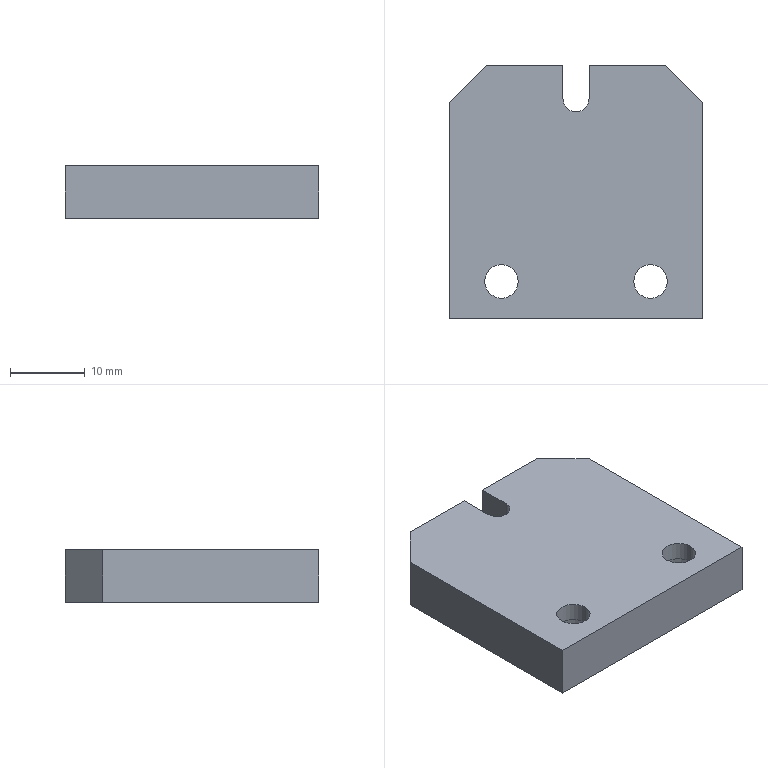Part | STEP file | 11-FG-B02011 | 1 solid | 22 faces | box 34 x 34 x 7 mm | volume 7241 mm3 | plane 13 | cylinder 9 | commonest cylinder face diameters 4.5 x4 8 x4 3.5 x1
STEP:
#1=CARTESIAN_POINT('',(11.,5.,4.5));
#2=VERTEX_POINT('',#1);
#3=CARTESIAN_POINT('',(3.,5.,4.5));
#4=VERTEX_POINT('',#3);
#5=CARTESIAN_POINT('',(7.,5.,4.5));
#6=DIRECTION('',(0.,0.,-1.));
#7=DIRECTION('',(-1.,0.,0.));
#8=AXIS2_PLACEMENT_3D('',#5,#6,#7);
#9=CIRCLE('',#8,4.);
#10=EDGE_CURVE('',#2,#4,#9,.T.);
#11=ORIENTED_EDGE('',*,*,#10,.F.);
#12=CARTESIAN_POINT('',(11.,5.,0.));
#13=VERTEX_POINT('',#12);
#14=CARTESIAN_POINT('',(11.,5.,4.5));
#15=DIRECTION('',(0.,0.,-1.));
#16=VECTOR('',#15,1000.);
#17=LINE('',#14,#16);
#18=EDGE_CURVE('',#2,#13,#17,.T.);
#19=ORIENTED_EDGE('',*,*,#18,.T.);
#20=CARTESIAN_POINT('',(3.,5.,0.));
#21=VERTEX_POINT('',#20);
#22=CARTESIAN_POINT('',(7.,5.,0.));
#23=DIRECTION('',(0.,0.,-1.));
#24=DIRECTION('',(-1.,0.,0.));
#25=AXIS2_PLACEMENT_3D('',#22,#23,#24);
#26=CIRCLE('',#25,4.);
#27=EDGE_CURVE('',#13,#21,#26,.T.);
#28=ORIENTED_EDGE('',*,*,#27,.T.);
#29=CARTESIAN_POINT('',(3.,5.,4.5));
#30=DIRECTION('',(0.,0.,-1.));
#31=VECTOR('',#30,1000.);
#32=LINE('',#29,#31);
#33=EDGE_CURVE('',#4,#21,#32,.T.);
#34=ORIENTED_EDGE('',*,*,#33,.F.);
#35=EDGE_LOOP('',(#11,#19,#28,#34));
#36=FACE_OUTER_BOUND('',#35,.T.);
#37=CARTESIAN_POINT('',(7.,5.,4.5));
#38=DIRECTION('',(0.,0.,-1.));
#39=DIRECTION('',(-1.,0.,0.));
#40=AXIS2_PLACEMENT_3D('',#37,#38,#39);
#41=CYLINDRICAL_SURFACE('',#40,4.);
#42=ADVANCED_FACE('',(#36),#41,.F.);
#43=CARTESIAN_POINT('',(31.,5.,4.5));
#44=VERTEX_POINT('',#43);
#45=CARTESIAN_POINT('',(23.,5.,4.5));
#46=VERTEX_POINT('',#45);
#47=CARTESIAN_POINT('',(27.,5.,4.5));
#48=DIRECTION('',(0.,0.,-1.));
#49=DIRECTION('',(-1.,0.,0.));
#50=AXIS2_PLACEMENT_3D('',#47,#48,#49);
#51=CIRCLE('',#50,4.);
#52=EDGE_CURVE('',#44,#46,#51,.T.);
#53=ORIENTED_EDGE('',*,*,#52,.F.);
#54=CARTESIAN_POINT('',(31.,5.,0.));
#55=VERTEX_POINT('',#54);
#56=CARTESIAN_POINT('',(31.,5.,4.5));
#57=DIRECTION('',(0.,0.,-1.));
#58=VECTOR('',#57,1000.);
#59=LINE('',#56,#58);
#60=EDGE_CURVE('',#44,#55,#59,.T.);
#61=ORIENTED_EDGE('',*,*,#60,.T.);
#62=CARTESIAN_POINT('',(23.,5.,0.));
#63=VERTEX_POINT('',#62);
#64=CARTESIAN_POINT('',(27.,5.,0.));
#65=DIRECTION('',(0.,0.,-1.));
#66=DIRECTION('',(-1.,0.,0.));
#67=AXIS2_PLACEMENT_3D('',#64,#65,#66);
#68=CIRCLE('',#67,4.);
#69=EDGE_CURVE('',#55,#63,#68,.T.);
#70=ORIENTED_EDGE('',*,*,#69,.T.);
#71=CARTESIAN_POINT('',(23.,5.,4.5));
#72=DIRECTION('',(0.,0.,-1.));
#73=VECTOR('',#72,1000.);
#74=LINE('',#71,#73);
#75=EDGE_CURVE('',#46,#63,#74,.T.);
#76=ORIENTED_EDGE('',*,*,#75,.F.);
#77=EDGE_LOOP('',(#53,#61,#70,#76));
#78=FACE_OUTER_BOUND('',#77,.T.);
#79=CARTESIAN_POINT('',(27.,5.,4.5));
#80=DIRECTION('',(0.,0.,-1.));
#81=DIRECTION('',(-1.,0.,0.));
#82=AXIS2_PLACEMENT_3D('',#79,#80,#81);
#83=CYLINDRICAL_SURFACE('',#82,4.);
#84=ADVANCED_FACE('',(#78),#83,.F.);
#85=CARTESIAN_POINT('',(24.75,5.,4.5));
#86=VERTEX_POINT('',#85);
#87=CARTESIAN_POINT('',(29.25,5.,4.5));
#88=VERTEX_POINT('',#87);
#89=CARTESIAN_POINT('',(27.,5.,4.5));
#90=DIRECTION('',(0.,0.,1.));
#91=DIRECTION('',(-1.,0.,0.));
#92=AXIS2_PLACEMENT_3D('',#89,#90,#91);
#93=CIRCLE('',#92,2.25);
#94=EDGE_CURVE('',#86,#88,#93,.T.);
#95=ORIENTED_EDGE('',*,*,#94,.F.);
#96=CARTESIAN_POINT('',(24.75,5.,7.));
#97=VERTEX_POINT('',#96);
#98=CARTESIAN_POINT('',(24.75,5.,0.));
#99=DIRECTION('',(0.,0.,1.));
#100=VECTOR('',#99,1000.);
#101=LINE('',#98,#100);
#102=EDGE_CURVE('',#86,#97,#101,.T.);
#103=ORIENTED_EDGE('',*,*,#102,.T.);
#104=CARTESIAN_POINT('',(29.25,5.,7.));
#105=VERTEX_POINT('',#104);
#106=CARTESIAN_POINT('',(27.,5.,7.));
#107=DIRECTION('',(0.,0.,1.));
#108=DIRECTION('',(1.,0.,0.));
#109=AXIS2_PLACEMENT_3D('',#106,#107,#108);
#110=CIRCLE('',#109,2.25);
#111=EDGE_CURVE('',#97,#105,#110,.T.);
#112=ORIENTED_EDGE('',*,*,#111,.T.);
#113=CARTESIAN_POINT('',(29.25,5.,0.));
#114=DIRECTION('',(0.,0.,1.));
#115=VECTOR('',#114,1000.);
#116=LINE('',#113,#115);
#117=EDGE_CURVE('',#88,#105,#116,.T.);
#118=ORIENTED_EDGE('',*,*,#117,.F.);
#119=EDGE_LOOP('',(#95,#103,#112,#118));
#120=FACE_OUTER_BOUND('',#119,.T.);
#121=CARTESIAN_POINT('',(27.,5.,0.));
#122=DIRECTION('',(0.,0.,1.));
#123=DIRECTION('',(1.,0.,0.));
#124=AXIS2_PLACEMENT_3D('',#121,#122,#123);
#125=CYLINDRICAL_SURFACE('',#124,2.25);
#126=ADVANCED_FACE('',(#120),#125,.F.);
#127=CARTESIAN_POINT('',(4.75,5.,4.5));
#128=VERTEX_POINT('',#127);
#129=CARTESIAN_POINT('',(9.25,5.,4.5));
#130=VERTEX_POINT('',#129);
#131=CARTESIAN_POINT('',(7.,5.,4.5));
#132=DIRECTION('',(0.,0.,1.));
#133=DIRECTION('',(-1.,0.,0.));
#134=AXIS2_PLACEMENT_3D('',#131,#132,#133);
#135=CIRCLE('',#134,2.25);
#136=EDGE_CURVE('',#128,#130,#135,.T.);
#137=ORIENTED_EDGE('',*,*,#136,.F.);
#138=CARTESIAN_POINT('',(4.75,5.,7.));
#139=VERTEX_POINT('',#138);
#140=CARTESIAN_POINT('',(4.75,5.,0.));
#141=DIRECTION('',(0.,0.,1.));
#142=VECTOR('',#141,1000.);
#143=LINE('',#140,#142);
#144=EDGE_CURVE('',#128,#139,#143,.T.);
#145=ORIENTED_EDGE('',*,*,#144,.T.);
#146=CARTESIAN_POINT('',(9.25,5.,7.));
#147=VERTEX_POINT('',#146);
#148=CARTESIAN_POINT('',(7.,5.,7.));
#149=DIRECTION('',(0.,0.,1.));
#150=DIRECTION('',(1.,0.,0.));
#151=AXIS2_PLACEMENT_3D('',#148,#149,#150);
#152=CIRCLE('',#151,2.25);
#153=EDGE_CURVE('',#139,#147,#152,.T.);
#154=ORIENTED_EDGE('',*,*,#153,.T.);
#155=CARTESIAN_POINT('',(9.25,5.,0.));
#156=DIRECTION('',(0.,0.,1.));
#157=VECTOR('',#156,1000.);
#158=LINE('',#155,#157);
#159=EDGE_CURVE('',#130,#147,#158,.T.);
#160=ORIENTED_EDGE('',*,*,#159,.F.);
#161=EDGE_LOOP('',(#137,#145,#154,#160));
#162=FACE_OUTER_BOUND('',#161,.T.);
#163=CARTESIAN_POINT('',(7.,5.,0.));
#164=DIRECTION('',(0.,0.,1.));
#165=DIRECTION('',(1.,0.,0.));
#166=AXIS2_PLACEMENT_3D('',#163,#164,#165);
#167=CYLINDRICAL_SURFACE('',#166,2.25);
#168=ADVANCED_FACE('',(#162),#167,.F.);
#169=ORIENTED_EDGE('',*,*,#144,.F.);
#170=CARTESIAN_POINT('',(7.,5.,4.5));
#171=DIRECTION('',(0.,0.,1.));
#172=DIRECTION('',(-1.,0.,0.));
#173=AXIS2_PLACEMENT_3D('',#170,#171,#172);
#174=CIRCLE('',#173,2.25);
#175=EDGE_CURVE('',#130,#128,#174,.T.);
#176=ORIENTED_EDGE('',*,*,#175,.F.);
#177=ORIENTED_EDGE('',*,*,#159,.T.);
#178=CARTESIAN_POINT('',(7.,5.,7.));
#179=DIRECTION('',(0.,0.,1.));
#180=DIRECTION('',(1.,0.,0.));
#181=AXIS2_PLACEMENT_3D('',#178,#179,#180);
#182=CIRCLE('',#181,2.25);
#183=EDGE_CURVE('',#147,#139,#182,.T.);
#184=ORIENTED_EDGE('',*,*,#183,.T.);
#185=EDGE_LOOP('',(#169,#176,#177,#184));
#186=FACE_OUTER_BOUND('',#185,.T.);
#187=CARTESIAN_POINT('',(7.,5.,0.));
#188=DIRECTION('',(0.,0.,1.));
#189=DIRECTION('',(1.,0.,0.));
#190=AXIS2_PLACEMENT_3D('',#187,#188,#189);
#191=CYLINDRICAL_SURFACE('',#190,2.25);
#192=ADVANCED_FACE('',(#186),#191,.F.);
#193=ORIENTED_EDGE('',*,*,#102,.F.);
#194=CARTESIAN_POINT('',(27.,5.,4.5));
#195=DIRECTION('',(0.,0.,1.));
#196=DIRECTION('',(-1.,0.,0.));
#197=AXIS2_PLACEMENT_3D('',#194,#195,#196);
#198=CIRCLE('',#197,2.25);
#199=EDGE_CURVE('',#88,#86,#198,.T.);
#200=ORIENTED_EDGE('',*,*,#199,.F.);
#201=ORIENTED_EDGE('',*,*,#117,.T.);
#202=CARTESIAN_POINT('',(27.,5.,7.));
#203=DIRECTION('',(0.,0.,1.));
#204=DIRECTION('',(1.,0.,0.));
#205=AXIS2_PLACEMENT_3D('',#202,#203,#204);
#206=CIRCLE('',#205,2.25);
#207=EDGE_CURVE('',#105,#97,#206,.T.);
#208=ORIENTED_EDGE('',*,*,#207,.T.);
#209=EDGE_LOOP('',(#193,#200,#201,#208));
#210=FACE_OUTER_BOUND('',#209,.T.);
#211=CARTESIAN_POINT('',(27.,5.,0.));
#212=DIRECTION('',(0.,0.,1.));
#213=DIRECTION('',(1.,0.,0.));
#214=AXIS2_PLACEMENT_3D('',#211,#212,#213);
#215=CYLINDRICAL_SURFACE('',#214,2.25);
#216=ADVANCED_FACE('',(#210),#215,.F.);
#217=CARTESIAN_POINT('',(29.,34.,0.));
#218=VERTEX_POINT('',#217);
#219=CARTESIAN_POINT('',(18.75,34.,0.));
#220=VERTEX_POINT('',#219);
#221=CARTESIAN_POINT('',(0.,34.,0.));
#222=DIRECTION('',(-1.,0.,0.));
#223=VECTOR('',#222,1000.);
#224=LINE('',#221,#223);
#225=EDGE_CURVE('',#218,#220,#224,.T.);
#226=ORIENTED_EDGE('',*,*,#225,.T.);
#227=CARTESIAN_POINT('',(18.75,34.,7.));
#228=VERTEX_POINT('',#227);
#229=CARTESIAN_POINT('',(18.75,34.,0.));
#230=DIRECTION('',(0.,0.,1.));
#231=VECTOR('',#230,1000.);
#232=LINE('',#229,#231);
#233=EDGE_CURVE('',#220,#228,#232,.T.);
#234=ORIENTED_EDGE('',*,*,#233,.T.);
#235=CARTESIAN_POINT('',(29.,34.,7.));
#236=VERTEX_POINT('',#235);
#237=CARTESIAN_POINT('',(0.,34.,7.));
#238=DIRECTION('',(-1.,0.,0.));
#239=VECTOR('',#238,1000.);
#240=LINE('',#237,#239);
#241=EDGE_CURVE('',#236,#228,#240,.T.);
#242=ORIENTED_EDGE('',*,*,#241,.F.);
#243=CARTESIAN_POINT('',(29.,34.,7.));
#244=DIRECTION('',(0.,0.,-1.));
#245=VECTOR('',#244,1000.);
#246=LINE('',#243,#245);
#247=EDGE_CURVE('',#236,#218,#246,.T.);
#248=ORIENTED_EDGE('',*,*,#247,.T.);
#249=EDGE_LOOP('',(#226,#234,#242,#248));
#250=FACE_OUTER_BOUND('',#249,.T.);
#251=CARTESIAN_POINT('',(0.,34.,7.));
#252=DIRECTION('',(0.,-1.,0.));
#253=DIRECTION('',(0.,0.,-1.));
#254=AXIS2_PLACEMENT_3D('',#251,#252,#253);
#255=PLANE('',#254);
#256=ADVANCED_FACE('',(#250),#255,.F.);
#257=CARTESIAN_POINT('',(0.,29.,7.));
#258=VERTEX_POINT('',#257);
#259=CARTESIAN_POINT('',(0.,0.,7.));
#260=VERTEX_POINT('',#259);
#261=CARTESIAN_POINT('',(0.,0.,7.));
#262=DIRECTION('',(0.,-1.,0.));
#263=VECTOR('',#262,1000.);
#264=LINE('',#261,#263);
#265=EDGE_CURVE('',#258,#260,#264,.T.);
#266=ORIENTED_EDGE('',*,*,#265,.F.);
#267=CARTESIAN_POINT('',(0.,29.,0.));
#268=VERTEX_POINT('',#267);
#269=CARTESIAN_POINT('',(0.,29.,7.));
#270=DIRECTION('',(0.,0.,-1.));
#271=VECTOR('',#270,1000.);
#272=LINE('',#269,#271);
#273=EDGE_CURVE('',#258,#268,#272,.T.);
#274=ORIENTED_EDGE('',*,*,#273,.T.);
#275=CARTESIAN_POINT('',(0.,0.,0.));
#276=VERTEX_POINT('',#275);
#277=CARTESIAN_POINT('',(0.,0.,0.));
#278=DIRECTION('',(0.,-1.,0.));
#279=VECTOR('',#278,1000.);
#280=LINE('',#277,#279);
#281=EDGE_CURVE('',#268,#276,#280,.T.);
#282=ORIENTED_EDGE('',*,*,#281,.T.);
#283=CARTESIAN_POINT('',(0.,0.,7.));
#284=DIRECTION('',(0.,0.,-1.));
#285=VECTOR('',#284,1000.);
#286=LINE('',#283,#285);
#287=EDGE_CURVE('',#260,#276,#286,.T.);
#288=ORIENTED_EDGE('',*,*,#287,.F.);
#289=EDGE_LOOP('',(#266,#274,#282,#288));
#290=FACE_OUTER_BOUND('',#289,.T.);
#291=CARTESIAN_POINT('',(0.,0.,7.));
#292=DIRECTION('',(1.,0.,0.));
#293=DIRECTION('',(0.,1.,0.));
#294=AXIS2_PLACEMENT_3D('',#291,#292,#293);
#295=PLANE('',#294);
#296=ADVANCED_FACE('',(#290),#295,.F.);
#297=CARTESIAN_POINT('',(34.,0.,0.));
#298=VERTEX_POINT('',#297);
#299=CARTESIAN_POINT('',(0.,0.,0.));
#300=DIRECTION('',(1.,0.,0.));
#301=VECTOR('',#300,1000.);
#302=LINE('',#299,#301);
#303=EDGE_CURVE('',#276,#298,#302,.T.);
#304=ORIENTED_EDGE('',*,*,#303,.T.);
#305=CARTESIAN_POINT('',(34.,0.,7.));
#306=VERTEX_POINT('',#305);
#307=CARTESIAN_POINT('',(34.,0.,7.));
#308=DIRECTION('',(0.,0.,-1.));
#309=VECTOR('',#308,1000.);
#310=LINE('',#307,#309);
#311=EDGE_CURVE('',#306,#298,#310,.T.);
#312=ORIENTED_EDGE('',*,*,#311,.F.);
#313=CARTESIAN_POINT('',(0.,0.,7.));
#314=DIRECTION('',(1.,0.,0.));
#315=VECTOR('',#314,1000.);
#316=LINE('',#313,#315);
#317=EDGE_CURVE('',#260,#306,#316,.T.);
#318=ORIENTED_EDGE('',*,*,#317,.F.);
#319=ORIENTED_EDGE('',*,*,#287,.T.);
#320=EDGE_LOOP('',(#304,#312,#318,#319));
#321=FACE_OUTER_BOUND('',#320,.T.);
#322=CARTESIAN_POINT('',(0.,0.,7.));
#323=DIRECTION('',(0.,1.,0.));
#324=DIRECTION('',(0.,0.,1.));
#325=AXIS2_PLACEMENT_3D('',#322,#323,#324);
#326=PLANE('',#325);
#327=ADVANCED_FACE('',(#321),#326,.F.);
#328=CARTESIAN_POINT('',(34.,29.,0.));
#329=VERTEX_POINT('',#328);
#330=CARTESIAN_POINT('',(34.,0.,0.));
#331=DIRECTION('',(0.,1.,0.));
#332=VECTOR('',#331,1000.);
#333=LINE('',#330,#332);
#334=EDGE_CURVE('',#298,#329,#333,.T.);
#335=ORIENTED_EDGE('',*,*,#334,.T.);
#336=CARTESIAN_POINT('',(34.,29.,7.));
#337=VERTEX_POINT('',#336);
#338=CARTESIAN_POINT('',(34.,29.,7.));
#339=DIRECTION('',(0.,0.,1.));
#340=VECTOR('',#339,1000.);
#341=LINE('',#338,#340);
#342=EDGE_CURVE('',#329,#337,#341,.T.);
#343=ORIENTED_EDGE('',*,*,#342,.T.);
#344=CARTESIAN_POINT('',(34.,0.,7.));
#345=DIRECTION('',(0.,1.,0.));
#346=VECTOR('',#345,1000.);
#347=LINE('',#344,#346);
#348=EDGE_CURVE('',#306,#337,#347,.T.);
#349=ORIENTED_EDGE('',*,*,#348,.F.);
#350=ORIENTED_EDGE('',*,*,#311,.T.);
#351=EDGE_LOOP('',(#335,#343,#349,#350));
#352=FACE_OUTER_BOUND('',#351,.T.);
#353=CARTESIAN_POINT('',(34.,0.,7.));
#354=DIRECTION('',(-1.,0.,0.));
#355=DIRECTION('',(0.,-1.,0.));
#356=AXIS2_PLACEMENT_3D('',#353,#354,#355);
#357=PLANE('',#356);
#358=ADVANCED_FACE('',(#352),#357,.F.);
#359=CARTESIAN_POINT('',(15.25,34.,7.));
#360=VERTEX_POINT('',#359);
#361=CARTESIAN_POINT('',(5.,34.,7.));
#362=VERTEX_POINT('',#361);
#363=CARTESIAN_POINT('',(0.,34.,7.));
#364=DIRECTION('',(-1.,0.,0.));
#365=VECTOR('',#364,1000.);
#366=LINE('',#363,#365);
#367=EDGE_CURVE('',#360,#362,#366,.T.);
#368=ORIENTED_EDGE('',*,*,#367,.F.);
#369=CARTESIAN_POINT('',(15.25,34.,0.));
#370=VERTEX_POINT('',#369);
#371=CARTESIAN_POINT('',(15.25,34.,0.));
#372=DIRECTION('',(0.,0.,1.));
#373=VECTOR('',#372,1000.);
#374=LINE('',#371,#373);
#375=EDGE_CURVE('',#370,#360,#374,.T.);
#376=ORIENTED_EDGE('',*,*,#375,.F.);
#377=CARTESIAN_POINT('',(5.,34.,0.));
#378=VERTEX_POINT('',#377);
#379=CARTESIAN_POINT('',(0.,34.,0.));
#380=DIRECTION('',(-1.,0.,0.));
#381=VECTOR('',#380,1000.);
#382=LINE('',#379,#381);
#383=EDGE_CURVE('',#370,#378,#382,.T.);
#384=ORIENTED_EDGE('',*,*,#383,.T.);
#385=CARTESIAN_POINT('',(5.,34.,7.));
#386=DIRECTION('',(0.,0.,1.));
#387=VECTOR('',#386,1000.);
#388=LINE('',#385,#387);
#389=EDGE_CURVE('',#378,#362,#388,.T.);
#390=ORIENTED_EDGE('',*,*,#389,.T.);
#391=EDGE_LOOP('',(#368,#376,#384,#390));
#392=FACE_OUTER_BOUND('',#391,.T.);
#393=CARTESIAN_POINT('',(0.,34.,7.));
#394=DIRECTION('',(0.,-1.,0.));
#395=DIRECTION('',(0.,0.,-1.));
#396=AXIS2_PLACEMENT_3D('',#393,#394,#395);
#397=PLANE('',#396);
#398=ADVANCED_FACE('',(#392),#397,.F.);
#399=ORIENTED_EDGE('',*,*,#207,.F.);
#400=ORIENTED_EDGE('',*,*,#111,.F.);
#401=EDGE_LOOP('',(#399,#400));
#402=FACE_BOUND('',#401,.T.);
#403=ORIENTED_EDGE('',*,*,#183,.F.);
#404=ORIENTED_EDGE('',*,*,#153,.F.);
#405=EDGE_LOOP('',(#403,#404));
#406=FACE_BOUND('',#405,.T.);
#407=ORIENTED_EDGE('',*,*,#241,.T.);
#408=CARTESIAN_POINT('',(18.75,29.5,7.));
#409=VERTEX_POINT('',#408);
#410=CARTESIAN_POINT('',(18.75,34.,7.));
#411=DIRECTION('',(0.,1.,0.));
#412=VECTOR('',#411,1000.);
#413=LINE('',#410,#412);
#414=EDGE_CURVE('',#409,#228,#413,.T.);
#415=ORIENTED_EDGE('',*,*,#414,.F.);
#416=CARTESIAN_POINT('',(15.25,29.5,7.));
#417=VERTEX_POINT('',#416);
#418=CARTESIAN_POINT('',(17.,29.5,7.));
#419=DIRECTION('',(0.,0.,1.));
#420=DIRECTION('',(1.,0.,0.));
#421=AXIS2_PLACEMENT_3D('',#418,#419,#420);
#422=CIRCLE('',#421,1.75);
#423=EDGE_CURVE('',#417,#409,#422,.T.);
#424=ORIENTED_EDGE('',*,*,#423,.F.);
#425=CARTESIAN_POINT('',(15.25,34.,7.));
#426=DIRECTION('',(0.,-1.,0.));
#427=VECTOR('',#426,1000.);
#428=LINE('',#425,#427);
#429=EDGE_CURVE('',#360,#417,#428,.T.);
#430=ORIENTED_EDGE('',*,*,#429,.F.);
#431=ORIENTED_EDGE('',*,*,#367,.T.);
#432=CARTESIAN_POINT('',(0.,29.,7.));
#433=DIRECTION('',(-0.7071,-0.7071,0.));
#434=VECTOR('',#433,1000.);
#435=LINE('',#432,#434);
#436=EDGE_CURVE('',#362,#258,#435,.T.);
#437=ORIENTED_EDGE('',*,*,#436,.T.);
#438=ORIENTED_EDGE('',*,*,#265,.T.);
#439=ORIENTED_EDGE('',*,*,#317,.T.);
#440=ORIENTED_EDGE('',*,*,#348,.T.);
#441=CARTESIAN_POINT('',(29.,34.,7.));
#442=DIRECTION('',(-0.7071,0.7071,0.));
#443=VECTOR('',#442,1000.);
#444=LINE('',#441,#443);
#445=EDGE_CURVE('',#337,#236,#444,.T.);
#446=ORIENTED_EDGE('',*,*,#445,.T.);
#447=EDGE_LOOP('',(#407,#415,#424,#430,#431,#437,#438,#439,#440,#446));
#448=FACE_OUTER_BOUND('',#447,.T.);
#449=CARTESIAN_POINT('',(0.,34.,7.));
#450=DIRECTION('',(0.,0.,-1.));
#451=DIRECTION('',(-1.,0.,0.));
#452=AXIS2_PLACEMENT_3D('',#449,#450,#451);
#453=PLANE('',#452);
#454=ADVANCED_FACE('',(#402,#406,#448),#453,.F.);
#455=CARTESIAN_POINT('',(7.,5.,0.));
#456=DIRECTION('',(0.,0.,-1.));
#457=DIRECTION('',(-1.,0.,0.));
#458=AXIS2_PLACEMENT_3D('',#455,#456,#457);
#459=CIRCLE('',#458,4.);
#460=EDGE_CURVE('',#21,#13,#459,.T.);
#461=ORIENTED_EDGE('',*,*,#460,.F.);
#462=ORIENTED_EDGE('',*,*,#27,.F.);
#463=EDGE_LOOP('',(#461,#462));
#464=FACE_BOUND('',#463,.T.);
#465=CARTESIAN_POINT('',(27.,5.,0.));
#466=DIRECTION('',(0.,0.,-1.));
#467=DIRECTION('',(-1.,0.,0.));
#468=AXIS2_PLACEMENT_3D('',#465,#466,#467);
#469=CIRCLE('',#468,4.);
#470=EDGE_CURVE('',#63,#55,#469,.T.);
#471=ORIENTED_EDGE('',*,*,#470,.F.);
#472=ORIENTED_EDGE('',*,*,#69,.F.);
#473=EDGE_LOOP('',(#471,#472));
#474=FACE_BOUND('',#473,.T.);
#475=CARTESIAN_POINT('',(18.75,29.5,0.));
#476=VERTEX_POINT('',#475);
#477=CARTESIAN_POINT('',(18.75,34.,0.));
#478=DIRECTION('',(0.,1.,0.));
#479=VECTOR('',#478,1000.);
#480=LINE('',#477,#479);
#481=EDGE_CURVE('',#476,#220,#480,.T.);
#482=ORIENTED_EDGE('',*,*,#481,.T.);
#483=ORIENTED_EDGE('',*,*,#225,.F.);
#484=CARTESIAN_POINT('',(14.5,48.5,0.));
#485=DIRECTION('',(0.7071,-0.7071,0.));
#486=VECTOR('',#485,1000.);
#487=LINE('',#484,#486);
#488=EDGE_CURVE('',#218,#329,#487,.T.);
#489=ORIENTED_EDGE('',*,*,#488,.T.);
#490=ORIENTED_EDGE('',*,*,#334,.F.);
#491=ORIENTED_EDGE('',*,*,#303,.F.);
#492=ORIENTED_EDGE('',*,*,#281,.F.);
#493=CARTESIAN_POINT('',(2.5,31.5,0.));
#494=DIRECTION('',(0.7071,0.7071,0.));
#495=VECTOR('',#494,1000.);
#496=LINE('',#493,#495);
#497=EDGE_CURVE('',#268,#378,#496,.T.);
#498=ORIENTED_EDGE('',*,*,#497,.T.);
#499=ORIENTED_EDGE('',*,*,#383,.F.);
#500=CARTESIAN_POINT('',(15.25,29.5,0.));
#501=VERTEX_POINT('',#500);
#502=CARTESIAN_POINT('',(15.25,34.,0.));
#503=DIRECTION('',(0.,-1.,0.));
#504=VECTOR('',#503,1000.);
#505=LINE('',#502,#504);
#506=EDGE_CURVE('',#370,#501,#505,.T.);
#507=ORIENTED_EDGE('',*,*,#506,.T.);
#508=CARTESIAN_POINT('',(17.,29.5,0.));
#509=DIRECTION('',(0.,0.,1.));
#510=DIRECTION('',(1.,0.,0.));
#511=AXIS2_PLACEMENT_3D('',#508,#509,#510);
#512=CIRCLE('',#511,1.75);
#513=EDGE_CURVE('',#501,#476,#512,.T.);
#514=ORIENTED_EDGE('',*,*,#513,.T.);
#515=EDGE_LOOP('',(#482,#483,#489,#490,#491,#492,#498,#499,#507,#514));
#516=FACE_OUTER_BOUND('',#515,.T.);
#517=CARTESIAN_POINT('',(0.,34.,0.));
#518=DIRECTION('',(0.,0.,-1.));
#519=DIRECTION('',(-1.,0.,0.));
#520=AXIS2_PLACEMENT_3D('',#517,#518,#519);
#521=PLANE('',#520);
#522=ADVANCED_FACE('',(#464,#474,#516),#521,.T.);
#523=ORIENTED_EDGE('',*,*,#436,.F.);
#524=ORIENTED_EDGE('',*,*,#389,.F.);
#525=ORIENTED_EDGE('',*,*,#497,.F.);
#526=ORIENTED_EDGE('',*,*,#273,.F.);
#527=EDGE_LOOP('',(#523,#524,#525,#526));
#528=FACE_OUTER_BOUND('',#527,.T.);
#529=CARTESIAN_POINT('',(0.,29.,7.));
#530=DIRECTION('',(0.7071,-0.7071,0.));
#531=DIRECTION('',(0.7071,0.7071,0.));
#532=AXIS2_PLACEMENT_3D('',#529,#530,#531);
#533=PLANE('',#532);
#534=ADVANCED_FACE('',(#528),#533,.F.);
#535=ORIENTED_EDGE('',*,*,#445,.F.);
#536=ORIENTED_EDGE('',*,*,#342,.F.);
#537=ORIENTED_EDGE('',*,*,#488,.F.);
#538=ORIENTED_EDGE('',*,*,#247,.F.);
#539=EDGE_LOOP('',(#535,#536,#537,#538));
#540=FACE_OUTER_BOUND('',#539,.T.);
#541=CARTESIAN_POINT('',(29.,34.,7.));
#542=DIRECTION('',(-0.7071,-0.7071,0.));
#543=DIRECTION('',(0.7071,-0.7071,0.));
#544=AXIS2_PLACEMENT_3D('',#541,#542,#543);
#545=PLANE('',#544);
#546=ADVANCED_FACE('',(#540),#545,.F.);
#547=ORIENTED_EDGE('',*,*,#414,.T.);
#548=ORIENTED_EDGE('',*,*,#233,.F.);
#549=ORIENTED_EDGE('',*,*,#481,.F.);
#550=CARTESIAN_POINT('',(18.75,29.5,0.));
#551=DIRECTION('',(0.,0.,1.));
#552=VECTOR('',#551,1000.);
#553=LINE('',#550,#552);
#554=EDGE_CURVE('',#476,#409,#553,.T.);
#555=ORIENTED_EDGE('',*,*,#554,.T.);
#556=EDGE_LOOP('',(#547,#548,#549,#555));
#557=FACE_OUTER_BOUND('',#556,.T.);
#558=CARTESIAN_POINT('',(18.75,34.,0.));
#559=DIRECTION('',(1.,0.,0.));
#560=DIRECTION('',(0.,0.,-1.));
#561=AXIS2_PLACEMENT_3D('',#558,#559,#560);
#562=PLANE('',#561);
#563=ADVANCED_FACE('',(#557),#562,.F.);
#564=ORIENTED_EDGE('',*,*,#423,.T.);
#565=ORIENTED_EDGE('',*,*,#554,.F.);
#566=ORIENTED_EDGE('',*,*,#513,.F.);
#567=CARTESIAN_POINT('',(15.25,29.5,0.));
#568=DIRECTION('',(0.,0.,1.));
#569=VECTOR('',#568,1000.);
#570=LINE('',#567,#569);
#571=EDGE_CURVE('',#501,#417,#570,.T.);
#572=ORIENTED_EDGE('',*,*,#571,.T.);
#573=EDGE_LOOP('',(#564,#565,#566,#572));
#574=FACE_OUTER_BOUND('',#573,.T.);
#575=CARTESIAN_POINT('',(17.,29.5,0.));
#576=DIRECTION('',(0.,0.,1.));
#577=DIRECTION('',(1.,0.,0.));
#578=AXIS2_PLACEMENT_3D('',#575,#576,#577);
#579=CYLINDRICAL_SURFACE('',#578,1.75);
#580=ADVANCED_FACE('',(#574),#579,.F.);
#581=ORIENTED_EDGE('',*,*,#429,.T.);
#582=ORIENTED_EDGE('',*,*,#571,.F.);
#583=ORIENTED_EDGE('',*,*,#506,.F.);
#584=ORIENTED_EDGE('',*,*,#375,.T.);
#585=EDGE_LOOP('',(#581,#582,#583,#584));
#586=FACE_OUTER_BOUND('',#585,.T.);
#587=CARTESIAN_POINT('',(15.25,34.,0.));
#588=DIRECTION('',(-1.,0.,0.));
#589=DIRECTION('',(0.,-1.,0.));
#590=AXIS2_PLACEMENT_3D('',#587,#588,#589);
#591=PLANE('',#590);
#592=ADVANCED_FACE('',(#586),#591,.F.);
#593=CARTESIAN_POINT('',(27.,5.,4.5));
#594=DIRECTION('',(0.,0.,-1.));
#595=DIRECTION('',(-1.,0.,0.));
#596=AXIS2_PLACEMENT_3D('',#593,#594,#595);
#597=CIRCLE('',#596,4.);
#598=EDGE_CURVE('',#46,#44,#597,.T.);
#599=ORIENTED_EDGE('',*,*,#598,.T.);
#600=ORIENTED_EDGE('',*,*,#52,.T.);
#601=EDGE_LOOP('',(#599,#600));
#602=FACE_OUTER_BOUND('',#601,.T.);
#603=ORIENTED_EDGE('',*,*,#199,.T.);
#604=ORIENTED_EDGE('',*,*,#94,.T.);
#605=EDGE_LOOP('',(#603,#604));
#606=FACE_BOUND('',#605,.T.);
#607=CARTESIAN_POINT('',(27.,5.,4.5));
#608=DIRECTION('',(0.,0.,-1.));
#609=DIRECTION('',(-1.,0.,0.));
#610=AXIS2_PLACEMENT_3D('',#607,#608,#609);
#611=PLANE('',#610);
#612=ADVANCED_FACE('',(#602,#606),#611,.T.);
#613=ORIENTED_EDGE('',*,*,#60,.F.);
#614=ORIENTED_EDGE('',*,*,#598,.F.);
#615=ORIENTED_EDGE('',*,*,#75,.T.);
#616=ORIENTED_EDGE('',*,*,#470,.T.);
#617=EDGE_LOOP('',(#613,#614,#615,#616));
#618=FACE_OUTER_BOUND('',#617,.T.);
#619=CARTESIAN_POINT('',(27.,5.,4.5));
#620=DIRECTION('',(0.,0.,-1.));
#621=DIRECTION('',(-1.,0.,0.));
#622=AXIS2_PLACEMENT_3D('',#619,#620,#621);
#623=CYLINDRICAL_SURFACE('',#622,4.);
#624=ADVANCED_FACE('',(#618),#623,.F.);
#625=CARTESIAN_POINT('',(7.,5.,4.5));
#626=DIRECTION('',(0.,0.,-1.));
#627=DIRECTION('',(-1.,0.,0.));
#628=AXIS2_PLACEMENT_3D('',#625,#626,#627);
#629=CIRCLE('',#628,4.);
#630=EDGE_CURVE('',#4,#2,#629,.T.);
#631=ORIENTED_EDGE('',*,*,#630,.T.);
#632=ORIENTED_EDGE('',*,*,#10,.T.);
#633=EDGE_LOOP('',(#631,#632));
#634=FACE_OUTER_BOUND('',#633,.T.);
#635=ORIENTED_EDGE('',*,*,#175,.T.);
#636=ORIENTED_EDGE('',*,*,#136,.T.);
#637=EDGE_LOOP('',(#635,#636));
#638=FACE_BOUND('',#637,.T.);
#639=CARTESIAN_POINT('',(7.,5.,4.5));
#640=DIRECTION('',(0.,0.,-1.));
#641=DIRECTION('',(-1.,0.,0.));
#642=AXIS2_PLACEMENT_3D('',#639,#640,#641);
#643=PLANE('',#642);
#644=ADVANCED_FACE('',(#634,#638),#643,.T.);
#645=ORIENTED_EDGE('',*,*,#18,.F.);
#646=ORIENTED_EDGE('',*,*,#630,.F.);
#647=ORIENTED_EDGE('',*,*,#33,.T.);
#648=ORIENTED_EDGE('',*,*,#460,.T.);
#649=EDGE_LOOP('',(#645,#646,#647,#648));
#650=FACE_OUTER_BOUND('',#649,.T.);
#651=CARTESIAN_POINT('',(7.,5.,4.5));
#652=DIRECTION('',(0.,0.,-1.));
#653=DIRECTION('',(-1.,0.,0.));
#654=AXIS2_PLACEMENT_3D('',#651,#652,#653);
#655=CYLINDRICAL_SURFACE('',#654,4.);
#656=ADVANCED_FACE('',(#650),#655,.F.);
#657=CLOSED_SHELL('',(#42,#84,#126,#168,#192,#216,#256,#296,#327,#358,#398,#454,#522,#534,#546,#563,#580,#592,#612,#624,#644,#656));
#658=MANIFOLD_SOLID_BREP('',#657);
#659=CARTESIAN_POINT('',(0.,0.,0.));
#660=DIRECTION('',(0.,0.,1.));
#661=DIRECTION('',(1.,0.,0.));
#662=AXIS2_PLACEMENT_3D('',#659,#660,#661);
#663=(LENGTH_UNIT()NAMED_UNIT(*)SI_UNIT(.MILLI.,.METRE.));
#664=UNCERTAINTY_MEASURE_WITH_UNIT(LENGTH_MEASURE(0.00001),#663,'','');
#665=(NAMED_UNIT(*)PLANE_ANGLE_UNIT()SI_UNIT($,.RADIAN.));
#666=(NAMED_UNIT(*)SI_UNIT($,.STERADIAN.)SOLID_ANGLE_UNIT());
#667=(GEOMETRIC_REPRESENTATION_CONTEXT(3)GLOBAL_UNCERTAINTY_ASSIGNED_CONTEXT((#664))GLOBAL_UNIT_ASSIGNED_CONTEXT((#663,#665,#666))REPRESENTATION_CONTEXT('',''));
#668=ADVANCED_BREP_SHAPE_REPRESENTATION('',(#658,#662),#667);